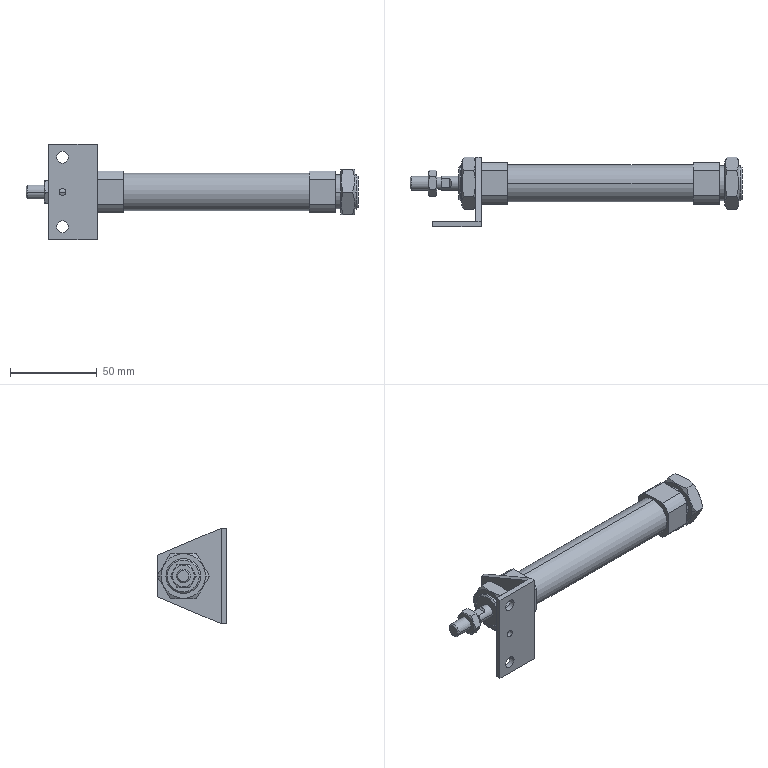Part | STEP file | CDM2L20-75Z_0_0_0_^Clamp cylinder assembly | 6 solids | 144 faces | box 191 x 40.011 x 55 mm | volume 57605 mm3 | plane 62 | cylinder 44 | cone 38 | commonest cylinder face diameters 20 x10 28 x8 8 x6 6.8 x4 8.566 x4 18.376 x4